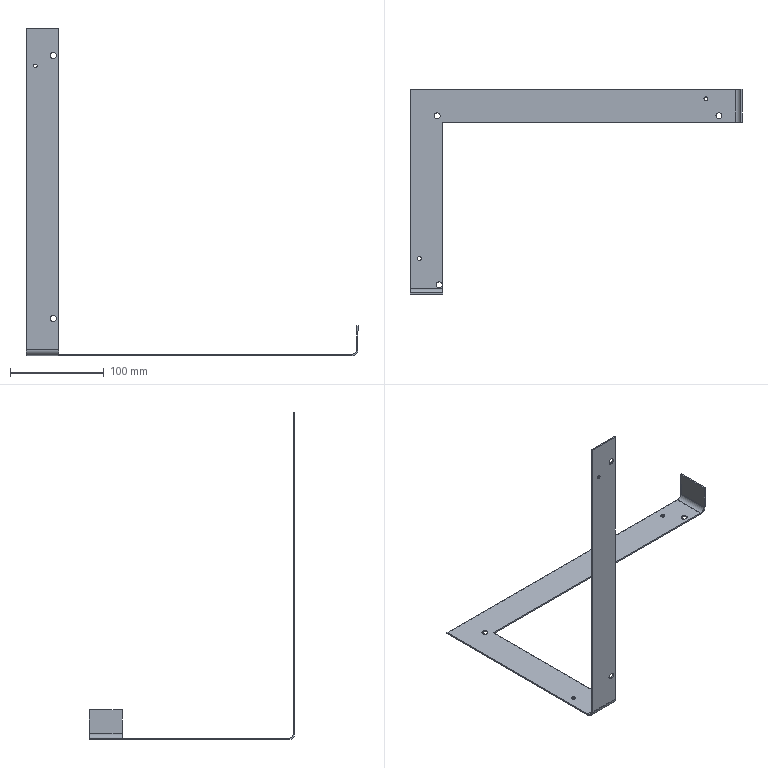Part | SolidWorks | features Cut 5, EdgeFlange 2, FlatPattern 1, SMBaseFlange 1, SheetMetal 1 | 1 solid | 40 faces | box 353.5 x 218.5 x 348.5 mm | volume 47454 mm3 | cylinder 20 | plane 20 | commonest cylinder face diameters 6.4 x10 4 x6 10 x2 13 x2
STEP:
#1=CARTESIAN_POINT('',(510.473,-27.361,-1.5));
#2=VERTEX_POINT('',#1);
#3=CARTESIAN_POINT('',(516.873,-27.361,-1.5));
#4=VERTEX_POINT('',#3);
#5=CARTESIAN_POINT('',(513.673,-27.361,-1.5));
#6=DIRECTION('',(0.,0.,1.));
#7=DIRECTION('',(1.,0.,0.));
#8=AXIS2_PLACEMENT_3D('',#5,#6,#7);
#9=CIRCLE('',#8,3.2);
#10=EDGE_CURVE('',#2,#4,#9,.T.);
#11=ORIENTED_EDGE('',*,*,#10,.F.);
#12=CARTESIAN_POINT('',(510.473,-27.361,0.));
#13=VERTEX_POINT('',#12);
#14=CARTESIAN_POINT('',(510.473,-27.361,-1.5));
#15=DIRECTION('',(0.,0.,1.));
#16=VECTOR('',#15,1000.);
#17=LINE('',#14,#16);
#18=EDGE_CURVE('',#2,#13,#17,.T.);
#19=ORIENTED_EDGE('',*,*,#18,.T.);
#20=CARTESIAN_POINT('',(516.873,-27.361,0.));
#21=VERTEX_POINT('',#20);
#22=CARTESIAN_POINT('',(513.673,-27.361,0.));
#23=DIRECTION('',(0.,0.,1.));
#24=DIRECTION('',(1.,0.,0.));
#25=AXIS2_PLACEMENT_3D('',#22,#23,#24);
#26=CIRCLE('',#25,3.2);
#27=EDGE_CURVE('',#13,#21,#26,.T.);
#28=ORIENTED_EDGE('',*,*,#27,.T.);
#29=CARTESIAN_POINT('',(516.873,-27.361,-1.5));
#30=DIRECTION('',(0.,0.,1.));
#31=VECTOR('',#30,1000.);
#32=LINE('',#29,#31);
#33=EDGE_CURVE('',#4,#21,#32,.T.);
#34=ORIENTED_EDGE('',*,*,#33,.F.);
#35=EDGE_LOOP('',(#11,#19,#28,#34));
#36=FACE_OUTER_BOUND('',#35,.T.);
#37=CARTESIAN_POINT('',(513.673,-27.361,-1.5));
#38=DIRECTION('',(0.,0.,1.));
#39=DIRECTION('',(1.,0.,0.));
#40=AXIS2_PLACEMENT_3D('',#37,#38,#39);
#41=CYLINDRICAL_SURFACE('',#40,3.2);
#42=ADVANCED_FACE('',(#36),#41,.F.);
#43=CARTESIAN_POINT('',(213.673,-217.715,314.8));
#44=VERTEX_POINT('',#43);
#45=CARTESIAN_POINT('',(213.673,-217.715,321.2));
#46=VERTEX_POINT('',#45);
#47=CARTESIAN_POINT('',(213.673,-217.715,318.));
#48=DIRECTION('',(0.,1.,0.));
#49=DIRECTION('',(0.,0.,1.));
#50=AXIS2_PLACEMENT_3D('',#47,#48,#49);
#51=CIRCLE('',#50,3.2);
#52=EDGE_CURVE('',#44,#46,#51,.T.);
#53=ORIENTED_EDGE('',*,*,#52,.F.);
#54=CARTESIAN_POINT('',(213.673,-216.215,314.8));
#55=VERTEX_POINT('',#54);
#56=CARTESIAN_POINT('',(213.673,-217.715,314.8));
#57=DIRECTION('',(0.,1.,0.));
#58=VECTOR('',#57,1000.);
#59=LINE('',#56,#58);
#60=EDGE_CURVE('',#44,#55,#59,.T.);
#61=ORIENTED_EDGE('',*,*,#60,.T.);
#62=CARTESIAN_POINT('',(213.673,-216.215,321.2));
#63=VERTEX_POINT('',#62);
#64=CARTESIAN_POINT('',(213.673,-216.215,318.));
#65=DIRECTION('',(0.,1.,0.));
#66=DIRECTION('',(0.,0.,1.));
#67=AXIS2_PLACEMENT_3D('',#64,#65,#66);
#68=CIRCLE('',#67,3.2);
#69=EDGE_CURVE('',#55,#63,#68,.T.);
#70=ORIENTED_EDGE('',*,*,#69,.T.);
#71=CARTESIAN_POINT('',(213.673,-217.715,321.2));
#72=DIRECTION('',(0.,1.,0.));
#73=VECTOR('',#72,1000.);
#74=LINE('',#71,#73);
#75=EDGE_CURVE('',#46,#63,#74,.T.);
#76=ORIENTED_EDGE('',*,*,#75,.F.);
#77=EDGE_LOOP('',(#53,#61,#70,#76));
#78=FACE_OUTER_BOUND('',#77,.T.);
#79=CARTESIAN_POINT('',(213.673,-217.715,318.));
#80=DIRECTION('',(0.,1.,0.));
#81=DIRECTION('',(0.,0.,1.));
#82=AXIS2_PLACEMENT_3D('',#79,#80,#81);
#83=CYLINDRICAL_SURFACE('',#82,3.2);
#84=ADVANCED_FACE('',(#78),#83,.F.);
#85=CARTESIAN_POINT('',(213.673,-217.715,34.8));
#86=VERTEX_POINT('',#85);
#87=CARTESIAN_POINT('',(213.673,-217.715,41.2));
#88=VERTEX_POINT('',#87);
#89=CARTESIAN_POINT('',(213.673,-217.715,38.));
#90=DIRECTION('',(0.,1.,0.));
#91=DIRECTION('',(0.,0.,1.));
#92=AXIS2_PLACEMENT_3D('',#89,#90,#91);
#93=CIRCLE('',#92,3.2);
#94=EDGE_CURVE('',#86,#88,#93,.T.);
#95=ORIENTED_EDGE('',*,*,#94,.F.);
#96=CARTESIAN_POINT('',(213.673,-216.215,34.8));
#97=VERTEX_POINT('',#96);
#98=CARTESIAN_POINT('',(213.673,-217.715,34.8));
#99=DIRECTION('',(0.,1.,0.));
#100=VECTOR('',#99,1000.);
#101=LINE('',#98,#100);
#102=EDGE_CURVE('',#86,#97,#101,.T.);
#103=ORIENTED_EDGE('',*,*,#102,.T.);
#104=CARTESIAN_POINT('',(213.673,-216.215,41.2));
#105=VERTEX_POINT('',#104);
#106=CARTESIAN_POINT('',(213.673,-216.215,38.));
#107=DIRECTION('',(0.,1.,0.));
#108=DIRECTION('',(0.,0.,1.));
#109=AXIS2_PLACEMENT_3D('',#106,#107,#108);
#110=CIRCLE('',#109,3.2);
#111=EDGE_CURVE('',#97,#105,#110,.T.);
#112=ORIENTED_EDGE('',*,*,#111,.T.);
#113=CARTESIAN_POINT('',(213.673,-217.715,41.2));
#114=DIRECTION('',(0.,1.,0.));
#115=VECTOR('',#114,1000.);
#116=LINE('',#113,#115);
#117=EDGE_CURVE('',#88,#105,#116,.T.);
#118=ORIENTED_EDGE('',*,*,#117,.F.);
#119=EDGE_LOOP('',(#95,#103,#112,#118));
#120=FACE_OUTER_BOUND('',#119,.T.);
#121=CARTESIAN_POINT('',(213.673,-217.715,38.));
#122=DIRECTION('',(0.,1.,0.));
#123=DIRECTION('',(0.,0.,1.));
#124=AXIS2_PLACEMENT_3D('',#121,#122,#123);
#125=CYLINDRICAL_SURFACE('',#124,3.2);
#126=ADVANCED_FACE('',(#120),#125,.F.);
#127=CARTESIAN_POINT('',(212.473,-207.35,-1.5));
#128=VERTEX_POINT('',#127);
#129=CARTESIAN_POINT('',(218.873,-207.35,-1.5));
#130=VERTEX_POINT('',#129);
#131=CARTESIAN_POINT('',(215.673,-207.35,-1.5));
#132=DIRECTION('',(0.,0.,1.));
#133=DIRECTION('',(1.,0.,0.));
#134=AXIS2_PLACEMENT_3D('',#131,#132,#133);
#135=CIRCLE('',#134,3.2);
#136=EDGE_CURVE('',#128,#130,#135,.T.);
#137=ORIENTED_EDGE('',*,*,#136,.F.);
#138=CARTESIAN_POINT('',(212.473,-207.35,0.));
#139=VERTEX_POINT('',#138);
#140=CARTESIAN_POINT('',(212.473,-207.35,-1.5));
#141=DIRECTION('',(0.,0.,1.));
#142=VECTOR('',#141,1000.);
#143=LINE('',#140,#142);
#144=EDGE_CURVE('',#128,#139,#143,.T.);
#145=ORIENTED_EDGE('',*,*,#144,.T.);
#146=CARTESIAN_POINT('',(218.873,-207.35,0.));
#147=VERTEX_POINT('',#146);
#148=CARTESIAN_POINT('',(215.673,-207.35,0.));
#149=DIRECTION('',(0.,0.,1.));
#150=DIRECTION('',(1.,0.,0.));
#151=AXIS2_PLACEMENT_3D('',#148,#149,#150);
#152=CIRCLE('',#151,3.2);
#153=EDGE_CURVE('',#139,#147,#152,.T.);
#154=ORIENTED_EDGE('',*,*,#153,.T.);
#155=CARTESIAN_POINT('',(218.873,-207.35,-1.5));
#156=DIRECTION('',(0.,0.,1.));
#157=VECTOR('',#156,1000.);
#158=LINE('',#155,#157);
#159=EDGE_CURVE('',#130,#147,#158,.T.);
#160=ORIENTED_EDGE('',*,*,#159,.F.);
#161=EDGE_LOOP('',(#137,#145,#154,#160));
#162=FACE_OUTER_BOUND('',#161,.T.);
#163=CARTESIAN_POINT('',(215.673,-207.35,-1.5));
#164=DIRECTION('',(0.,0.,1.));
#165=DIRECTION('',(1.,0.,0.));
#166=AXIS2_PLACEMENT_3D('',#163,#164,#165);
#167=CYLINDRICAL_SURFACE('',#166,3.2);
#168=ADVANCED_FACE('',(#162),#167,.F.);
#169=CARTESIAN_POINT('',(210.473,-27.361,-1.5));
#170=VERTEX_POINT('',#169);
#171=CARTESIAN_POINT('',(216.873,-27.361,-1.5));
#172=VERTEX_POINT('',#171);
#173=CARTESIAN_POINT('',(213.673,-27.361,-1.5));
#174=DIRECTION('',(0.,0.,1.));
#175=DIRECTION('',(1.,0.,0.));
#176=AXIS2_PLACEMENT_3D('',#173,#174,#175);
#177=CIRCLE('',#176,3.2);
#178=EDGE_CURVE('',#170,#172,#177,.T.);
#179=ORIENTED_EDGE('',*,*,#178,.F.);
#180=CARTESIAN_POINT('',(210.473,-27.361,0.));
#181=VERTEX_POINT('',#180);
#182=CARTESIAN_POINT('',(210.473,-27.361,-1.5));
#183=DIRECTION('',(0.,0.,1.));
#184=VECTOR('',#183,1000.);
#185=LINE('',#182,#184);
#186=EDGE_CURVE('',#170,#181,#185,.T.);
#187=ORIENTED_EDGE('',*,*,#186,.T.);
#188=CARTESIAN_POINT('',(216.873,-27.361,0.));
#189=VERTEX_POINT('',#188);
#190=CARTESIAN_POINT('',(213.673,-27.361,0.));
#191=DIRECTION('',(0.,0.,1.));
#192=DIRECTION('',(1.,0.,0.));
#193=AXIS2_PLACEMENT_3D('',#190,#191,#192);
#194=CIRCLE('',#193,3.2);
#195=EDGE_CURVE('',#181,#189,#194,.T.);
#196=ORIENTED_EDGE('',*,*,#195,.T.);
#197=CARTESIAN_POINT('',(216.873,-27.361,-1.5));
#198=DIRECTION('',(0.,0.,1.));
#199=VECTOR('',#198,1000.);
#200=LINE('',#197,#199);
#201=EDGE_CURVE('',#172,#189,#200,.T.);
#202=ORIENTED_EDGE('',*,*,#201,.F.);
#203=EDGE_LOOP('',(#179,#187,#196,#202));
#204=FACE_OUTER_BOUND('',#203,.T.);
#205=CARTESIAN_POINT('',(213.673,-27.361,-1.5));
#206=DIRECTION('',(0.,0.,1.));
#207=DIRECTION('',(1.,0.,0.));
#208=AXIS2_PLACEMENT_3D('',#205,#206,#207);
#209=CYLINDRICAL_SURFACE('',#208,3.2);
#210=ADVANCED_FACE('',(#204),#209,.F.);
#211=CARTESIAN_POINT('',(194.673,-216.215,305.));
#212=VERTEX_POINT('',#211);
#213=CARTESIAN_POINT('',(194.673,-216.215,309.));
#214=VERTEX_POINT('',#213);
#215=CARTESIAN_POINT('',(194.673,-216.215,307.));
#216=DIRECTION('',(0.,1.,0.));
#217=DIRECTION('',(0.,0.,1.));
#218=AXIS2_PLACEMENT_3D('',#215,#216,#217);
#219=CIRCLE('',#218,2.);
#220=EDGE_CURVE('',#212,#214,#219,.T.);
#221=ORIENTED_EDGE('',*,*,#220,.T.);
#222=CARTESIAN_POINT('',(194.673,-217.715,309.));
#223=VERTEX_POINT('',#222);
#224=CARTESIAN_POINT('',(194.673,-207.715,309.));
#225=DIRECTION('',(0.,-1.,0.));
#226=VECTOR('',#225,1000.);
#227=LINE('',#224,#226);
#228=EDGE_CURVE('',#214,#223,#227,.T.);
#229=ORIENTED_EDGE('',*,*,#228,.T.);
#230=CARTESIAN_POINT('',(194.673,-217.715,305.));
#231=VERTEX_POINT('',#230);
#232=CARTESIAN_POINT('',(194.673,-217.715,307.));
#233=DIRECTION('',(0.,-1.,0.));
#234=DIRECTION('',(0.,0.,-1.));
#235=AXIS2_PLACEMENT_3D('',#232,#233,#234);
#236=CIRCLE('',#235,2.);
#237=EDGE_CURVE('',#223,#231,#236,.T.);
#238=ORIENTED_EDGE('',*,*,#237,.T.);
#239=CARTESIAN_POINT('',(194.673,-207.715,305.));
#240=DIRECTION('',(0.,-1.,0.));
#241=VECTOR('',#240,1000.);
#242=LINE('',#239,#241);
#243=EDGE_CURVE('',#212,#231,#242,.T.);
#244=ORIENTED_EDGE('',*,*,#243,.F.);
#245=EDGE_LOOP('',(#221,#229,#238,#244));
#246=FACE_OUTER_BOUND('',#245,.T.);
#247=CARTESIAN_POINT('',(194.673,-207.715,307.));
#248=DIRECTION('',(0.,-1.,0.));
#249=DIRECTION('',(0.,0.,-1.));
#250=AXIS2_PLACEMENT_3D('',#247,#248,#249);
#251=CYLINDRICAL_SURFACE('',#250,2.);
#252=ADVANCED_FACE('',(#246),#251,.F.);
#253=CARTESIAN_POINT('',(497.673,-9.215,0.));
#254=VERTEX_POINT('',#253);
#255=CARTESIAN_POINT('',(501.673,-9.215,0.));
#256=VERTEX_POINT('',#255);
#257=CARTESIAN_POINT('',(499.673,-9.215,0.));
#258=DIRECTION('',(0.,0.,1.));
#259=DIRECTION('',(1.,0.,0.));
#260=AXIS2_PLACEMENT_3D('',#257,#258,#259);
#261=CIRCLE('',#260,2.);
#262=EDGE_CURVE('',#254,#256,#261,.T.);
#263=ORIENTED_EDGE('',*,*,#262,.T.);
#264=CARTESIAN_POINT('',(501.673,-9.215,-1.5));
#265=VERTEX_POINT('',#264);
#266=CARTESIAN_POINT('',(501.673,-9.215,8.5));
#267=DIRECTION('',(0.,0.,-1.));
#268=VECTOR('',#267,1000.);
#269=LINE('',#266,#268);
#270=EDGE_CURVE('',#256,#265,#269,.T.);
#271=ORIENTED_EDGE('',*,*,#270,.T.);
#272=CARTESIAN_POINT('',(497.673,-9.215,-1.5));
#273=VERTEX_POINT('',#272);
#274=CARTESIAN_POINT('',(499.673,-9.215,-1.5));
#275=DIRECTION('',(0.,0.,-1.));
#276=DIRECTION('',(-1.,0.,0.));
#277=AXIS2_PLACEMENT_3D('',#274,#275,#276);
#278=CIRCLE('',#277,2.);
#279=EDGE_CURVE('',#265,#273,#278,.T.);
#280=ORIENTED_EDGE('',*,*,#279,.T.);
#281=CARTESIAN_POINT('',(497.673,-9.215,8.5));
#282=DIRECTION('',(0.,0.,-1.));
#283=VECTOR('',#282,1000.);
#284=LINE('',#281,#283);
#285=EDGE_CURVE('',#254,#273,#284,.T.);
#286=ORIENTED_EDGE('',*,*,#285,.F.);
#287=EDGE_LOOP('',(#263,#271,#280,#286));
#288=FACE_OUTER_BOUND('',#287,.T.);
#289=CARTESIAN_POINT('',(499.673,-9.215,8.5));
#290=DIRECTION('',(0.,0.,-1.));
#291=DIRECTION('',(-1.,0.,0.));
#292=AXIS2_PLACEMENT_3D('',#289,#290,#291);
#293=CYLINDRICAL_SURFACE('',#292,2.);
#294=ADVANCED_FACE('',(#288),#293,.F.);
#295=CARTESIAN_POINT('',(192.673,-179.215,0.));
#296=VERTEX_POINT('',#295);
#297=CARTESIAN_POINT('',(196.673,-179.215,0.));
#298=VERTEX_POINT('',#297);
#299=CARTESIAN_POINT('',(194.673,-179.215,0.));
#300=DIRECTION('',(0.,0.,1.));
#301=DIRECTION('',(1.,0.,0.));
#302=AXIS2_PLACEMENT_3D('',#299,#300,#301);
#303=CIRCLE('',#302,2.);
#304=EDGE_CURVE('',#296,#298,#303,.T.);
#305=ORIENTED_EDGE('',*,*,#304,.T.);
#306=CARTESIAN_POINT('',(196.673,-179.215,-1.5));
#307=VERTEX_POINT('',#306);
#308=CARTESIAN_POINT('',(196.673,-179.215,8.5));
#309=DIRECTION('',(0.,0.,-1.));
#310=VECTOR('',#309,1000.);
#311=LINE('',#308,#310);
#312=EDGE_CURVE('',#298,#307,#311,.T.);
#313=ORIENTED_EDGE('',*,*,#312,.T.);
#314=CARTESIAN_POINT('',(192.673,-179.215,-1.5));
#315=VERTEX_POINT('',#314);
#316=CARTESIAN_POINT('',(194.673,-179.215,-1.5));
#317=DIRECTION('',(0.,0.,-1.));
#318=DIRECTION('',(-1.,0.,0.));
#319=AXIS2_PLACEMENT_3D('',#316,#317,#318);
#320=CIRCLE('',#319,2.);
#321=EDGE_CURVE('',#307,#315,#320,.T.);
#322=ORIENTED_EDGE('',*,*,#321,.T.);
#323=CARTESIAN_POINT('',(192.673,-179.215,8.5));
#324=DIRECTION('',(0.,0.,-1.));
#325=VECTOR('',#324,1000.);
#326=LINE('',#323,#325);
#327=EDGE_CURVE('',#296,#315,#326,.T.);
#328=ORIENTED_EDGE('',*,*,#327,.F.);
#329=EDGE_LOOP('',(#305,#313,#322,#328));
#330=FACE_OUTER_BOUND('',#329,.T.);
#331=CARTESIAN_POINT('',(194.673,-179.215,8.5));
#332=DIRECTION('',(0.,0.,-1.));
#333=DIRECTION('',(-1.,0.,0.));
#334=AXIS2_PLACEMENT_3D('',#331,#332,#333);
#335=CYLINDRICAL_SURFACE('',#334,2.);
#336=ADVANCED_FACE('',(#330),#335,.F.);
#337=CARTESIAN_POINT('',(513.673,-27.361,-1.5));
#338=DIRECTION('',(0.,0.,1.));
#339=DIRECTION('',(1.,0.,0.));
#340=AXIS2_PLACEMENT_3D('',#337,#338,#339);
#341=CIRCLE('',#340,3.2);
#342=EDGE_CURVE('',#4,#2,#341,.T.);
#343=ORIENTED_EDGE('',*,*,#342,.T.);
#344=ORIENTED_EDGE('',*,*,#10,.T.);
#345=EDGE_LOOP('',(#343,#344));
#346=FACE_BOUND('',#345,.T.);
#347=CARTESIAN_POINT('',(215.673,-207.35,-1.5));
#348=DIRECTION('',(0.,0.,1.));
#349=DIRECTION('',(1.,0.,0.));
#350=AXIS2_PLACEMENT_3D('',#347,#348,#349);
#351=CIRCLE('',#350,3.2);
#352=EDGE_CURVE('',#130,#128,#351,.T.);
#353=ORIENTED_EDGE('',*,*,#352,.T.);
#354=ORIENTED_EDGE('',*,*,#136,.T.);
#355=EDGE_LOOP('',(#353,#354));
#356=FACE_BOUND('',#355,.T.);
#357=CARTESIAN_POINT('',(213.673,-27.361,-1.5));
#358=DIRECTION('',(0.,0.,1.));
#359=DIRECTION('',(1.,0.,0.));
#360=AXIS2_PLACEMENT_3D('',#357,#358,#359);
#361=CIRCLE('',#360,3.2);
#362=EDGE_CURVE('',#172,#170,#361,.T.);
#363=ORIENTED_EDGE('',*,*,#362,.T.);
#364=ORIENTED_EDGE('',*,*,#178,.T.);
#365=EDGE_LOOP('',(#363,#364));
#366=FACE_BOUND('',#365,.T.);
#367=CARTESIAN_POINT('',(499.673,-9.215,-1.5));
#368=DIRECTION('',(0.,0.,-1.));
#369=DIRECTION('',(-1.,0.,0.));
#370=AXIS2_PLACEMENT_3D('',#367,#368,#369);
#371=CIRCLE('',#370,2.);
#372=EDGE_CURVE('',#273,#265,#371,.T.);
#373=ORIENTED_EDGE('',*,*,#372,.F.);
#374=ORIENTED_EDGE('',*,*,#279,.F.);
#375=EDGE_LOOP('',(#373,#374));
#376=FACE_BOUND('',#375,.T.);
#377=CARTESIAN_POINT('',(194.673,-179.215,-1.5));
#378=DIRECTION('',(0.,0.,-1.));
#379=DIRECTION('',(-1.,0.,0.));
#380=AXIS2_PLACEMENT_3D('',#377,#378,#379);
#381=CIRCLE('',#380,2.);
#382=EDGE_CURVE('',#315,#307,#381,.T.);
#383=ORIENTED_EDGE('',*,*,#382,.F.);
#384=ORIENTED_EDGE('',*,*,#321,.F.);
#385=EDGE_LOOP('',(#383,#384));
#386=FACE_BOUND('',#385,.T.);
#387=CARTESIAN_POINT('',(531.673,0.7853,-1.5));
#388=VERTEX_POINT('',#387);
#389=CARTESIAN_POINT('',(531.673,-34.215,-1.5));
#390=VERTEX_POINT('',#389);
#391=CARTESIAN_POINT('',(531.673,0.7853,-1.5));
#392=DIRECTION('',(0.,-1.,0.));
#393=VECTOR('',#392,1000.);
#394=LINE('',#391,#393);
#395=EDGE_CURVE('',#388,#390,#394,.T.);
#396=ORIENTED_EDGE('',*,*,#395,.T.);
#397=CARTESIAN_POINT('',(219.673,-34.215,-1.5));
#398=VERTEX_POINT('',#397);
#399=CARTESIAN_POINT('',(219.673,-34.215,-1.5));
#400=DIRECTION('',(1.,0.,0.));
#401=VECTOR('',#400,1000.);
#402=LINE('',#399,#401);
#403=EDGE_CURVE('',#398,#390,#402,.T.);
#404=ORIENTED_EDGE('',*,*,#403,.F.);
#405=CARTESIAN_POINT('',(219.673,-211.215,-1.5));
#406=VERTEX_POINT('',#405);
#407=CARTESIAN_POINT('',(219.673,-34.215,-1.5));
#408=DIRECTION('',(0.,1.,0.));
#409=VECTOR('',#408,1000.);
#410=LINE('',#407,#409);
#411=EDGE_CURVE('',#406,#398,#410,.T.);
#412=ORIENTED_EDGE('',*,*,#411,.F.);
#413=CARTESIAN_POINT('',(184.673,-211.215,-1.5));
#414=VERTEX_POINT('',#413);
#415=CARTESIAN_POINT('',(219.673,-211.215,-1.5));
#416=DIRECTION('',(-1.,0.,0.));
#417=VECTOR('',#416,1000.);
#418=LINE('',#415,#417);
#419=EDGE_CURVE('',#406,#414,#418,.T.);
#420=ORIENTED_EDGE('',*,*,#419,.T.);
#421=CARTESIAN_POINT('',(184.673,0.7853,-1.5));
#422=VERTEX_POINT('',#421);
#423=CARTESIAN_POINT('',(184.673,0.7853,-1.5));
#424=DIRECTION('',(0.,-1.,0.));
#425=VECTOR('',#424,1000.);
#426=LINE('',#423,#425);
#427=EDGE_CURVE('',#422,#414,#426,.T.);
#428=ORIENTED_EDGE('',*,*,#427,.F.);
#429=CARTESIAN_POINT('',(184.673,0.7853,-1.5));
#430=DIRECTION('',(-1.,0.,0.));
#431=VECTOR('',#430,1000.);
#432=LINE('',#429,#431);
#433=EDGE_CURVE('',#388,#422,#432,.T.);
#434=ORIENTED_EDGE('',*,*,#433,.F.);
#435=EDGE_LOOP('',(#396,#404,#412,#420,#428,#434));
#436=FACE_OUTER_BOUND('',#435,.T.);
#437=CARTESIAN_POINT('',(0.,0.,-1.5));
#438=DIRECTION('',(0.,0.,1.));
#439=DIRECTION('',(1.,0.,0.));
#440=AXIS2_PLACEMENT_3D('',#437,#438,#439);
#441=PLANE('',#440);
#442=ADVANCED_FACE('',(#346,#356,#366,#376,#386,#436),#441,.F.);
#443=CARTESIAN_POINT('',(513.673,-27.361,0.));
#444=DIRECTION('',(0.,0.,1.));
#445=DIRECTION('',(1.,0.,0.));
#446=AXIS2_PLACEMENT_3D('',#443,#444,#445);
#447=CIRCLE('',#446,3.2);
#448=EDGE_CURVE('',#21,#13,#447,.T.);
#449=ORIENTED_EDGE('',*,*,#448,.F.);
#450=ORIENTED_EDGE('',*,*,#27,.F.);
#451=EDGE_LOOP('',(#449,#450));
#452=FACE_BOUND('',#451,.T.);
#453=CARTESIAN_POINT('',(215.673,-207.35,0.));
#454=DIRECTION('',(0.,0.,1.));
#455=DIRECTION('',(1.,0.,0.));
#456=AXIS2_PLACEMENT_3D('',#453,#454,#455);
#457=CIRCLE('',#456,3.2);
#458=EDGE_CURVE('',#147,#139,#457,.T.);
#459=ORIENTED_EDGE('',*,*,#458,.F.);
#460=ORIENTED_EDGE('',*,*,#153,.F.);
#461=EDGE_LOOP('',(#459,#460));
#462=FACE_BOUND('',#461,.T.);
#463=CARTESIAN_POINT('',(213.673,-27.361,0.));
#464=DIRECTION('',(0.,0.,1.));
#465=DIRECTION('',(1.,0.,0.));
#466=AXIS2_PLACEMENT_3D('',#463,#464,#465);
#467=CIRCLE('',#466,3.2);
#468=EDGE_CURVE('',#189,#181,#467,.T.);
#469=ORIENTED_EDGE('',*,*,#468,.F.);
#470=ORIENTED_EDGE('',*,*,#195,.F.);
#471=EDGE_LOOP('',(#469,#470));
#472=FACE_BOUND('',#471,.T.);
#473=ORIENTED_EDGE('',*,*,#262,.F.);
#474=CARTESIAN_POINT('',(499.673,-9.215,0.));
#475=DIRECTION('',(0.,0.,1.));
#476=DIRECTION('',(1.,0.,0.));
#477=AXIS2_PLACEMENT_3D('',#474,#475,#476);
#478=CIRCLE('',#477,2.);
#479=EDGE_CURVE('',#256,#254,#478,.T.);
#480=ORIENTED_EDGE('',*,*,#479,.F.);
#481=EDGE_LOOP('',(#473,#480));
#482=FACE_BOUND('',#481,.T.);
#483=ORIENTED_EDGE('',*,*,#304,.F.);
#484=CARTESIAN_POINT('',(194.673,-179.215,0.));
#485=DIRECTION('',(0.,0.,1.));
#486=DIRECTION('',(1.,0.,0.));
#487=AXIS2_PLACEMENT_3D('',#484,#485,#486);
#488=CIRCLE('',#487,2.);
#489=EDGE_CURVE('',#298,#296,#488,.T.);
#490=ORIENTED_EDGE('',*,*,#489,.F.);
#491=EDGE_LOOP('',(#483,#490));
#492=FACE_BOUND('',#491,.T.);
#493=CARTESIAN_POINT('',(219.673,-34.215,0.));
#494=VERTEX_POINT('',#493);
#495=CARTESIAN_POINT('',(531.673,-34.215,0.));
#496=VERTEX_POINT('',#495);
#497=CARTESIAN_POINT('',(219.673,-34.215,0.));
#498=DIRECTION('',(1.,0.,0.));
#499=VECTOR('',#498,1000.);
#500=LINE('',#497,#499);
#501=EDGE_CURVE('',#494,#496,#500,.T.);
#502=ORIENTED_EDGE('',*,*,#501,.T.);
#503=CARTESIAN_POINT('',(531.673,0.7853,0.));
#504=VERTEX_POINT('',#503);
#505=CARTESIAN_POINT('',(531.673,0.7853,0.));
#506=DIRECTION('',(0.,-1.,0.));
#507=VECTOR('',#506,1000.);
#508=LINE('',#505,#507);
#509=EDGE_CURVE('',#504,#496,#508,.T.);
#510=ORIENTED_EDGE('',*,*,#509,.F.);
#511=CARTESIAN_POINT('',(184.673,0.7853,0.));
#512=VERTEX_POINT('',#511);
#513=CARTESIAN_POINT('',(184.673,0.7853,0.));
#514=DIRECTION('',(-1.,0.,0.));
#515=VECTOR('',#514,1000.);
#516=LINE('',#513,#515);
#517=EDGE_CURVE('',#504,#512,#516,.T.);
#518=ORIENTED_EDGE('',*,*,#517,.T.);
#519=CARTESIAN_POINT('',(184.673,-211.215,0.));
#520=VERTEX_POINT('',#519);
#521=CARTESIAN_POINT('',(184.673,0.7853,0.));
#522=DIRECTION('',(0.,-1.,0.));
#523=VECTOR('',#522,1000.);
#524=LINE('',#521,#523);
#525=EDGE_CURVE('',#512,#520,#524,.T.);
#526=ORIENTED_EDGE('',*,*,#525,.T.);
#527=CARTESIAN_POINT('',(219.673,-211.215,0.));
#528=VERTEX_POINT('',#527);
#529=CARTESIAN_POINT('',(219.673,-211.215,0.));
#530=DIRECTION('',(-1.,0.,0.));
#531=VECTOR('',#530,1000.);
#532=LINE('',#529,#531);
#533=EDGE_CURVE('',#528,#520,#532,.T.);
#534=ORIENTED_EDGE('',*,*,#533,.F.);
#535=CARTESIAN_POINT('',(219.673,-34.215,0.));
#536=DIRECTION('',(0.,1.,0.));
#537=VECTOR('',#536,1000.);
#538=LINE('',#535,#537);
#539=EDGE_CURVE('',#528,#494,#538,.T.);
#540=ORIENTED_EDGE('',*,*,#539,.T.);
#541=EDGE_LOOP('',(#502,#510,#518,#526,#534,#540));
#542=FACE_OUTER_BOUND('',#541,.T.);
#543=CARTESIAN_POINT('',(0.,0.,0.));
#544=DIRECTION('',(0.,0.,1.));
#545=DIRECTION('',(1.,0.,0.));
#546=AXIS2_PLACEMENT_3D('',#543,#544,#545);
#547=PLANE('',#546);
#548=ADVANCED_FACE('',(#452,#462,#472,#482,#492,#542),#547,.T.);
#549=ORIENTED_EDGE('',*,*,#517,.F.);
#550=CARTESIAN_POINT('',(531.673,0.7853,0.));
#551=DIRECTION('',(0.,0.,-1.));
#552=VECTOR('',#551,1000.);
#553=LINE('',#550,#552);
#554=EDGE_CURVE('',#504,#388,#553,.T.);
#555=ORIENTED_EDGE('',*,*,#554,.T.);
#556=ORIENTED_EDGE('',*,*,#433,.T.);
#557=CARTESIAN_POINT('',(184.673,0.7853,-1.5));
#558=DIRECTION('',(0.,0.,1.));
#559=VECTOR('',#558,1000.);
#560=LINE('',#557,#559);
#561=EDGE_CURVE('',#422,#512,#560,.T.);
#562=ORIENTED_EDGE('',*,*,#561,.T.);
#563=EDGE_LOOP('',(#549,#555,#556,#562));
#564=FACE_OUTER_BOUND('',#563,.T.);
#565=CARTESIAN_POINT('',(184.673,0.7853,-1.5));
#566=DIRECTION('',(0.,1.,0.));
#567=DIRECTION('',(0.,0.,1.));
#568=AXIS2_PLACEMENT_3D('',#565,#566,#567);
#569=PLANE('',#568);
#570=ADVANCED_FACE('',(#564),#569,.T.);
#571=ORIENTED_EDGE('',*,*,#539,.F.);
#572=CARTESIAN_POINT('',(219.673,-211.215,0.));
#573=DIRECTION('',(0.,0.,-1.));
#574=VECTOR('',#573,1000.);
#575=LINE('',#572,#574);
#576=EDGE_CURVE('',#528,#406,#575,.T.);
#577=ORIENTED_EDGE('',*,*,#576,.T.);
#578=ORIENTED_EDGE('',*,*,#411,.T.);
#579=CARTESIAN_POINT('',(219.673,-34.215,-1.5));
#580=DIRECTION('',(0.,0.,1.));
#581=VECTOR('',#580,1000.);
#582=LINE('',#579,#581);
#583=EDGE_CURVE('',#398,#494,#582,.T.);
#584=ORIENTED_EDGE('',*,*,#583,.T.);
#585=EDGE_LOOP('',(#571,#577,#578,#584));
#586=FACE_OUTER_BOUND('',#585,.T.);
#587=CARTESIAN_POINT('',(219.673,-34.215,-1.5));
#588=DIRECTION('',(1.,0.,0.));
#589=DIRECTION('',(0.,1.,0.));
#590=AXIS2_PLACEMENT_3D('',#587,#588,#589);
#591=PLANE('',#590);
#592=ADVANCED_FACE('',(#586),#591,.T.);
#593=CARTESIAN_POINT('',(184.673,-211.215,0.));
#594=DIRECTION('',(0.,0.,-1.));
#595=VECTOR('',#594,1000.);
#596=LINE('',#593,#595);
#597=EDGE_CURVE('',#520,#414,#596,.T.);
#598=ORIENTED_EDGE('',*,*,#597,.F.);
#599=ORIENTED_EDGE('',*,*,#525,.F.);
#600=ORIENTED_EDGE('',*,*,#561,.F.);
#601=ORIENTED_EDGE('',*,*,#427,.T.);
#602=EDGE_LOOP('',(#598,#599,#600,#601));
#603=FACE_OUTER_BOUND('',#602,.T.);
#604=CARTESIAN_POINT('',(184.673,0.7853,-1.5));
#605=DIRECTION('',(-1.,0.,0.));
#606=DIRECTION('',(0.,-1.,0.));
#607=AXIS2_PLACEMENT_3D('',#604,#605,#606);
#608=PLANE('',#607);
#609=ADVANCED_FACE('',(#603),#608,.T.);
#610=CARTESIAN_POINT('',(531.673,-34.215,0.));
#611=DIRECTION('',(0.,0.,-1.));
#612=VECTOR('',#611,1000.);
#613=LINE('',#610,#612);
#614=EDGE_CURVE('',#496,#390,#613,.T.);
#615=ORIENTED_EDGE('',*,*,#614,.F.);
#616=ORIENTED_EDGE('',*,*,#501,.F.);
#617=ORIENTED_EDGE('',*,*,#583,.F.);
#618=ORIENTED_EDGE('',*,*,#403,.T.);
#619=EDGE_LOOP('',(#615,#616,#617,#618));
#620=FACE_OUTER_BOUND('',#619,.T.);
#621=CARTESIAN_POINT('',(219.673,-34.215,-1.5));
#622=DIRECTION('',(0.,-1.,0.));
#623=DIRECTION('',(0.,0.,-1.));
#624=AXIS2_PLACEMENT_3D('',#621,#622,#623);
#625=PLANE('',#624);
#626=ADVANCED_FACE('',(#620),#625,.T.);
#627=CARTESIAN_POINT('',(184.673,-216.215,5.));
#628=VERTEX_POINT('',#627);
#629=CARTESIAN_POINT('',(184.673,-217.715,5.));
#630=VERTEX_POINT('',#629);
#631=CARTESIAN_POINT('',(184.673,-217.715,5.));
#632=DIRECTION('',(0.,-1.,0.));
#633=VECTOR('',#632,1000.);
#634=LINE('',#631,#633);
#635=EDGE_CURVE('',#628,#630,#634,.T.);
#636=ORIENTED_EDGE('',*,*,#635,.F.);
#637=CARTESIAN_POINT('',(184.673,-211.215,5.));
#638=DIRECTION('',(-1.,0.,0.));
#639=DIRECTION('',(0.,0.,-1.));
#640=AXIS2_PLACEMENT_3D('',#637,#638,#639);
#641=CIRCLE('',#640,5.);
#642=EDGE_CURVE('',#520,#628,#641,.T.);
#643=ORIENTED_EDGE('',*,*,#642,.F.);
#644=ORIENTED_EDGE('',*,*,#597,.T.);
#645=CARTESIAN_POINT('',(184.673,-211.215,5.));
#646=DIRECTION('',(-1.,0.,0.));
#647=DIRECTION('',(0.,0.,-1.));
#648=AXIS2_PLACEMENT_3D('',#645,#646,#647);
#649=CIRCLE('',#648,6.5);
#650=EDGE_CURVE('',#414,#630,#649,.T.);
#651=ORIENTED_EDGE('',*,*,#650,.T.);
#652=EDGE_LOOP('',(#636,#643,#644,#651));
#653=FACE_OUTER_BOUND('',#652,.T.);
#654=CARTESIAN_POINT('',(184.673,-211.215,5.));
#655=DIRECTION('',(-1.,0.,0.));
#656=DIRECTION('',(0.,0.,1.));
#657=AXIS2_PLACEMENT_3D('',#654,#655,#656);
#658=PLANE('',#657);
#659=ADVANCED_FACE('',(#653),#658,.T.);
#660=CARTESIAN_POINT('',(219.673,-216.215,5.));
#661=VERTEX_POINT('',#660);
#662=CARTESIAN_POINT('',(219.673,-211.215,5.));
#663=DIRECTION('',(1.,0.,0.));
#664=DIRECTION('',(0.,0.,-1.));
#665=AXIS2_PLACEMENT_3D('',#662,#663,#664);
#666=CIRCLE('',#665,5.);
#667=EDGE_CURVE('',#661,#528,#666,.T.);
#668=ORIENTED_EDGE('',*,*,#667,.F.);
#669=CARTESIAN_POINT('',(219.673,-217.715,5.));
#670=VERTEX_POINT('',#669);
#671=CARTESIAN_POINT('',(219.673,-216.215,5.));
#672=DIRECTION('',(0.,-1.,0.));
#673=VECTOR('',#672,1000.);
#674=LINE('',#671,#673);
#675=EDGE_CURVE('',#661,#670,#674,.T.);
#676=ORIENTED_EDGE('',*,*,#675,.T.);
#677=CARTESIAN_POINT('',(219.673,-211.215,5.));
#678=DIRECTION('',(1.,0.,0.));
#679=DIRECTION('',(0.,0.,-1.));
#680=AXIS2_PLACEMENT_3D('',#677,#678,#679);
#681=CIRCLE('',#680,6.5);
#682=EDGE_CURVE('',#670,#406,#681,.T.);
#683=ORIENTED_EDGE('',*,*,#682,.T.);
#684=ORIENTED_EDGE('',*,*,#576,.F.);
#685=EDGE_LOOP('',(#668,#676,#683,#684));
#686=FACE_OUTER_BOUND('',#685,.T.);
#687=CARTESIAN_POINT('',(219.673,-211.215,5.));
#688=DIRECTION('',(-1.,0.,0.));
#689=DIRECTION('',(0.,0.,1.));
#690=AXIS2_PLACEMENT_3D('',#687,#688,#689);
#691=PLANE('',#690);
#692=ADVANCED_FACE('',(#686),#691,.F.);
#693=ORIENTED_EDGE('',*,*,#419,.F.);
#694=ORIENTED_EDGE('',*,*,#682,.F.);
#695=CARTESIAN_POINT('',(184.673,-217.715,5.));
#696=DIRECTION('',(-1.,0.,0.));
#697=VECTOR('',#696,1000.);
#698=LINE('',#695,#697);
#699=EDGE_CURVE('',#670,#630,#698,.T.);
#700=ORIENTED_EDGE('',*,*,#699,.T.);
#701=ORIENTED_EDGE('',*,*,#650,.F.);
#702=EDGE_LOOP('',(#693,#694,#700,#701));
#703=FACE_OUTER_BOUND('',#702,.T.);
#704=CARTESIAN_POINT('',(219.673,-211.215,5.));
#705=DIRECTION('',(1.,0.,0.));
#706=DIRECTION('',(0.,-1.,0.));
#707=AXIS2_PLACEMENT_3D('',#704,#705,#706);
#708=CYLINDRICAL_SURFACE('',#707,6.5);
#709=ADVANCED_FACE('',(#703),#708,.T.);
#710=ORIENTED_EDGE('',*,*,#533,.T.);
#711=ORIENTED_EDGE('',*,*,#642,.T.);
#712=CARTESIAN_POINT('',(184.673,-216.215,5.));
#713=DIRECTION('',(1.,0.,0.));
#714=VECTOR('',#713,1000.);
#715=LINE('',#712,#714);
#716=EDGE_CURVE('',#628,#661,#715,.T.);
#717=ORIENTED_EDGE('',*,*,#716,.T.);
#718=ORIENTED_EDGE('',*,*,#667,.T.);
#719=EDGE_LOOP('',(#710,#711,#717,#718));
#720=FACE_OUTER_BOUND('',#719,.T.);
#721=CARTESIAN_POINT('',(219.673,-211.215,5.));
#722=DIRECTION('',(1.,0.,0.));
#723=DIRECTION('',(0.,-1.,0.));
#724=AXIS2_PLACEMENT_3D('',#721,#722,#723);
#725=CYLINDRICAL_SURFACE('',#724,5.);
#726=ADVANCED_FACE('',(#720),#725,.F.);
#727=ORIENTED_EDGE('',*,*,#675,.F.);
#728=CARTESIAN_POINT('',(219.673,-216.215,347.));
#729=VERTEX_POINT('',#728);
#730=CARTESIAN_POINT('',(219.673,-216.215,347.));
#731=DIRECTION('',(0.,0.,1.));
#732=VECTOR('',#731,1000.);
#733=LINE('',#730,#732);
#734=EDGE_CURVE('',#661,#729,#733,.T.);
#735=ORIENTED_EDGE('',*,*,#734,.T.);
#736=CARTESIAN_POINT('',(219.673,-217.715,347.));
#737=VERTEX_POINT('',#736);
#738=CARTESIAN_POINT('',(219.673,-217.715,347.));
#739=DIRECTION('',(0.,1.,0.));
#740=VECTOR('',#739,1000.);
#741=LINE('',#738,#740);
#742=EDGE_CURVE('',#737,#729,#741,.T.);
#743=ORIENTED_EDGE('',*,*,#742,.F.);
#744=CARTESIAN_POINT('',(219.673,-217.715,0.));
#745=DIRECTION('',(0.,0.,1.));
#746=VECTOR('',#745,1000.);
#747=LINE('',#744,#746);
#748=EDGE_CURVE('',#670,#737,#747,.T.);
#749=ORIENTED_EDGE('',*,*,#748,.F.);
#750=EDGE_LOOP('',(#727,#735,#743,#749));
#751=FACE_OUTER_BOUND('',#750,.T.);
#752=CARTESIAN_POINT('',(219.673,-217.715,347.));
#753=DIRECTION('',(-1.,0.,0.));
#754=DIRECTION('',(0.,0.,1.));
#755=AXIS2_PLACEMENT_3D('',#752,#753,#754);
#756=PLANE('',#755);
#757=ADVANCED_FACE('',(#751),#756,.F.);
#758=ORIENTED_EDGE('',*,*,#635,.T.);
#759=CARTESIAN_POINT('',(184.673,-217.715,347.));
#760=VERTEX_POINT('',#759);
#761=CARTESIAN_POINT('',(184.673,-217.715,0.));
#762=DIRECTION('',(0.,0.,-1.));
#763=VECTOR('',#762,1000.);
#764=LINE('',#761,#763);
#765=EDGE_CURVE('',#760,#630,#764,.T.);
#766=ORIENTED_EDGE('',*,*,#765,.F.);
#767=CARTESIAN_POINT('',(184.673,-216.215,347.));
#768=VERTEX_POINT('',#767);
#769=CARTESIAN_POINT('',(184.673,-217.715,347.));
#770=DIRECTION('',(0.,1.,0.));
#771=VECTOR('',#770,1000.);
#772=LINE('',#769,#771);
#773=EDGE_CURVE('',#760,#768,#772,.T.);
#774=ORIENTED_EDGE('',*,*,#773,.T.);
#775=CARTESIAN_POINT('',(184.673,-216.215,0.));
#776=DIRECTION('',(0.,0.,-1.));
#777=VECTOR('',#776,1000.);
#778=LINE('',#775,#777);
#779=EDGE_CURVE('',#768,#628,#778,.T.);
#780=ORIENTED_EDGE('',*,*,#779,.T.);
#781=EDGE_LOOP('',(#758,#766,#774,#780));
#782=FACE_OUTER_BOUND('',#781,.T.);
#783=CARTESIAN_POINT('',(184.673,-217.715,0.));
#784=DIRECTION('',(1.,0.,0.));
#785=DIRECTION('',(0.,0.,-1.));
#786=AXIS2_PLACEMENT_3D('',#783,#784,#785);
#787=PLANE('',#786);
#788=ADVANCED_FACE('',(#782),#787,.F.);
#789=CARTESIAN_POINT('',(213.673,-217.715,318.));
#790=DIRECTION('',(0.,1.,0.));
#791=DIRECTION('',(0.,0.,1.));
#792=AXIS2_PLACEMENT_3D('',#789,#790,#791);
#793=CIRCLE('',#792,3.2);
#794=EDGE_CURVE('',#46,#44,#793,.T.);
#795=ORIENTED_EDGE('',*,*,#794,.T.);
#796=ORIENTED_EDGE('',*,*,#52,.T.);
#797=EDGE_LOOP('',(#795,#796));
#798=FACE_BOUND('',#797,.T.);
#799=CARTESIAN_POINT('',(213.673,-217.715,38.));
#800=DIRECTION('',(0.,1.,0.));
#801=DIRECTION('',(0.,0.,1.));
#802=AXIS2_PLACEMENT_3D('',#799,#800,#801);
#803=CIRCLE('',#802,3.2);
#804=EDGE_CURVE('',#88,#86,#803,.T.);
#805=ORIENTED_EDGE('',*,*,#804,.T.);
#806=ORIENTED_EDGE('',*,*,#94,.T.);
#807=EDGE_LOOP('',(#805,#806));
#808=FACE_BOUND('',#807,.T.);
#809=CARTESIAN_POINT('',(194.673,-217.715,307.));
#810=DIRECTION('',(0.,-1.,0.));
#811=DIRECTION('',(0.,0.,-1.));
#812=AXIS2_PLACEMENT_3D('',#809,#810,#811);
#813=CIRCLE('',#812,2.);
#814=EDGE_CURVE('',#231,#223,#813,.T.);
#815=ORIENTED_EDGE('',*,*,#814,.F.);
#816=ORIENTED_EDGE('',*,*,#237,.F.);
#817=EDGE_LOOP('',(#815,#816));
#818=FACE_BOUND('',#817,.T.);
#819=ORIENTED_EDGE('',*,*,#699,.F.);
#820=ORIENTED_EDGE('',*,*,#748,.T.);
#821=CARTESIAN_POINT('',(0.,-217.715,347.));
#822=DIRECTION('',(-1.,0.,0.));
#823=VECTOR('',#822,1000.);
#824=LINE('',#821,#823);
#825=EDGE_CURVE('',#737,#760,#824,.T.);
#826=ORIENTED_EDGE('',*,*,#825,.T.);
#827=ORIENTED_EDGE('',*,*,#765,.T.);
#828=EDGE_LOOP('',(#819,#820,#826,#827));
#829=FACE_OUTER_BOUND('',#828,.T.);
#830=CARTESIAN_POINT('',(0.,-217.715,0.));
#831=DIRECTION('',(0.,1.,0.));
#832=DIRECTION('',(0.,0.,1.));
#833=AXIS2_PLACEMENT_3D('',#830,#831,#832);
#834=PLANE('',#833);
#835=ADVANCED_FACE('',(#798,#808,#818,#829),#834,.F.);
#836=CARTESIAN_POINT('',(213.673,-216.215,318.));
#837=DIRECTION('',(0.,1.,0.));
#838=DIRECTION('',(0.,0.,1.));
#839=AXIS2_PLACEMENT_3D('',#836,#837,#838);
#840=CIRCLE('',#839,3.2);
#841=EDGE_CURVE('',#63,#55,#840,.T.);
#842=ORIENTED_EDGE('',*,*,#841,.F.);
#843=ORIENTED_EDGE('',*,*,#69,.F.);
#844=EDGE_LOOP('',(#842,#843));
#845=FACE_BOUND('',#844,.T.);
#846=CARTESIAN_POINT('',(213.673,-216.215,38.));
#847=DIRECTION('',(0.,1.,0.));
#848=DIRECTION('',(0.,0.,1.));
#849=AXIS2_PLACEMENT_3D('',#846,#847,#848);
#850=CIRCLE('',#849,3.2);
#851=EDGE_CURVE('',#105,#97,#850,.T.);
#852=ORIENTED_EDGE('',*,*,#851,.F.);
#853=ORIENTED_EDGE('',*,*,#111,.F.);
#854=EDGE_LOOP('',(#852,#853));
#855=FACE_BOUND('',#854,.T.);
#856=ORIENTED_EDGE('',*,*,#220,.F.);
#857=CARTESIAN_POINT('',(194.673,-216.215,307.));
#858=DIRECTION('',(0.,1.,0.));
#859=DIRECTION('',(0.,0.,1.));
#860=AXIS2_PLACEMENT_3D('',#857,#858,#859);
#861=CIRCLE('',#860,2.);
#862=EDGE_CURVE('',#214,#212,#861,.T.);
#863=ORIENTED_EDGE('',*,*,#862,.F.);
#864=EDGE_LOOP('',(#856,#863));
#865=FACE_BOUND('',#864,.T.);
#866=ORIENTED_EDGE('',*,*,#734,.F.);
#867=ORIENTED_EDGE('',*,*,#716,.F.);
#868=ORIENTED_EDGE('',*,*,#779,.F.);
#869=CARTESIAN_POINT('',(184.673,-216.215,347.));
#870=DIRECTION('',(-1.,0.,0.));
#871=VECTOR('',#870,1000.);
#872=LINE('',#869,#871);
#873=EDGE_CURVE('',#729,#768,#872,.T.);
#874=ORIENTED_EDGE('',*,*,#873,.F.);
#875=EDGE_LOOP('',(#866,#867,#868,#874));
#876=FACE_OUTER_BOUND('',#875,.T.);
#877=CARTESIAN_POINT('',(0.,-216.215,0.));
#878=DIRECTION('',(0.,1.,0.));
#879=DIRECTION('',(0.,0.,1.));
#880=AXIS2_PLACEMENT_3D('',#877,#878,#879);
#881=PLANE('',#880);
#882=ADVANCED_FACE('',(#845,#855,#865,#876),#881,.T.);
#883=ORIENTED_EDGE('',*,*,#873,.T.);
#884=ORIENTED_EDGE('',*,*,#773,.F.);
#885=ORIENTED_EDGE('',*,*,#825,.F.);
#886=ORIENTED_EDGE('',*,*,#742,.T.);
#887=EDGE_LOOP('',(#883,#884,#885,#886));
#888=FACE_OUTER_BOUND('',#887,.T.);
#889=CARTESIAN_POINT('',(184.673,-217.715,347.));
#890=DIRECTION('',(0.,0.,-1.));
#891=DIRECTION('',(0.,1.,0.));
#892=AXIS2_PLACEMENT_3D('',#889,#890,#891);
#893=PLANE('',#892);
#894=ADVANCED_FACE('',(#888),#893,.F.);
#895=CARTESIAN_POINT('',(536.673,-34.215,5.));
#896=VERTEX_POINT('',#895);
#897=CARTESIAN_POINT('',(538.173,-34.215,5.));
#898=VERTEX_POINT('',#897);
#899=CARTESIAN_POINT('',(538.173,-34.215,5.));
#900=DIRECTION('',(1.,0.,0.));
#901=VECTOR('',#900,1000.);
#902=LINE('',#899,#901);
#903=EDGE_CURVE('',#896,#898,#902,.T.);
#904=ORIENTED_EDGE('',*,*,#903,.F.);
#905=CARTESIAN_POINT('',(531.673,-34.215,5.));
#906=DIRECTION('',(0.,-1.,0.));
#907=DIRECTION('',(0.,0.,1.));
#908=AXIS2_PLACEMENT_3D('',#905,#906,#907);
#909=CIRCLE('',#908,5.);
#910=EDGE_CURVE('',#496,#896,#909,.T.);
#911=ORIENTED_EDGE('',*,*,#910,.F.);
#912=ORIENTED_EDGE('',*,*,#614,.T.);
#913=CARTESIAN_POINT('',(531.673,-34.215,5.));
#914=DIRECTION('',(0.,-1.,0.));
#915=DIRECTION('',(0.,0.,1.));
#916=AXIS2_PLACEMENT_3D('',#913,#914,#915);
#917=CIRCLE('',#916,6.5);
#918=EDGE_CURVE('',#390,#898,#917,.T.);
#919=ORIENTED_EDGE('',*,*,#918,.T.);
#920=EDGE_LOOP('',(#904,#911,#912,#919));
#921=FACE_OUTER_BOUND('',#920,.T.);
#922=CARTESIAN_POINT('',(531.673,-34.215,5.));
#923=DIRECTION('',(0.,-1.,0.));
#924=DIRECTION('',(0.,0.,-1.));
#925=AXIS2_PLACEMENT_3D('',#922,#923,#924);
#926=PLANE('',#925);
#927=ADVANCED_FACE('',(#921),#926,.T.);
#928=CARTESIAN_POINT('',(536.673,0.7853,5.));
#929=VERTEX_POINT('',#928);
#930=CARTESIAN_POINT('',(531.673,0.7853,5.));
#931=DIRECTION('',(0.,1.,0.));
#932=DIRECTION('',(0.,0.,1.));
#933=AXIS2_PLACEMENT_3D('',#930,#931,#932);
#934=CIRCLE('',#933,5.);
#935=EDGE_CURVE('',#929,#504,#934,.T.);
#936=ORIENTED_EDGE('',*,*,#935,.F.);
#937=CARTESIAN_POINT('',(538.173,0.7853,5.));
#938=VERTEX_POINT('',#937);
#939=CARTESIAN_POINT('',(536.673,0.7853,5.));
#940=DIRECTION('',(1.,0.,0.));
#941=VECTOR('',#940,1000.);
#942=LINE('',#939,#941);
#943=EDGE_CURVE('',#929,#938,#942,.T.);
#944=ORIENTED_EDGE('',*,*,#943,.T.);
#945=CARTESIAN_POINT('',(531.673,0.7853,5.));
#946=DIRECTION('',(0.,1.,0.));
#947=DIRECTION('',(0.,0.,1.));
#948=AXIS2_PLACEMENT_3D('',#945,#946,#947);
#949=CIRCLE('',#948,6.5);
#950=EDGE_CURVE('',#938,#388,#949,.T.);
#951=ORIENTED_EDGE('',*,*,#950,.T.);
#952=ORIENTED_EDGE('',*,*,#554,.F.);
#953=EDGE_LOOP('',(#936,#944,#951,#952));
#954=FACE_OUTER_BOUND('',#953,.T.);
#955=CARTESIAN_POINT('',(531.673,0.7853,5.));
#956=DIRECTION('',(0.,-1.,0.));
#957=DIRECTION('',(0.,0.,-1.));
#958=AXIS2_PLACEMENT_3D('',#955,#956,#957);
#959=PLANE('',#958);
#960=ADVANCED_FACE('',(#954),#959,.F.);
#961=ORIENTED_EDGE('',*,*,#395,.F.);
#962=ORIENTED_EDGE('',*,*,#950,.F.);
#963=CARTESIAN_POINT('',(538.173,0.,5.));
#964=DIRECTION('',(0.,1.,0.));
#965=VECTOR('',#964,1000.);
#966=LINE('',#963,#965);
#967=EDGE_CURVE('',#898,#938,#966,.T.);
#968=ORIENTED_EDGE('',*,*,#967,.F.);
#969=ORIENTED_EDGE('',*,*,#918,.F.);
#970=EDGE_LOOP('',(#961,#962,#968,#969));
#971=FACE_OUTER_BOUND('',#970,.T.);
#972=CARTESIAN_POINT('',(531.673,0.7853,5.));
#973=DIRECTION('',(0.,1.,0.));
#974=DIRECTION('',(1.,0.,0.));
#975=AXIS2_PLACEMENT_3D('',#972,#973,#974);
#976=CYLINDRICAL_SURFACE('',#975,6.5);
#977=ADVANCED_FACE('',(#971),#976,.T.);
#978=ORIENTED_EDGE('',*,*,#509,.T.);
#979=ORIENTED_EDGE('',*,*,#910,.T.);
#980=CARTESIAN_POINT('',(536.673,-34.215,5.));
#981=DIRECTION('',(0.,1.,0.));
#982=VECTOR('',#981,1000.);
#983=LINE('',#980,#982);
#984=EDGE_CURVE('',#896,#929,#983,.T.);
#985=ORIENTED_EDGE('',*,*,#984,.T.);
#986=ORIENTED_EDGE('',*,*,#935,.T.);
#987=EDGE_LOOP('',(#978,#979,#985,#986));
#988=FACE_OUTER_BOUND('',#987,.T.);
#989=CARTESIAN_POINT('',(531.673,0.7853,5.));
#990=DIRECTION('',(0.,1.,0.));
#991=DIRECTION('',(1.,0.,0.));
#992=AXIS2_PLACEMENT_3D('',#989,#990,#991);
#993=CYLINDRICAL_SURFACE('',#992,5.);
#994=ADVANCED_FACE('',(#988),#993,.F.);
#995=CARTESIAN_POINT('',(538.173,0.7853,30.5));
#996=VERTEX_POINT('',#995);
#997=CARTESIAN_POINT('',(538.173,0.7853,0.));
#998=DIRECTION('',(0.,0.,-1.));
#999=VECTOR('',#998,1000.);
#1000=LINE('',#997,#999);
#1001=EDGE_CURVE('',#996,#938,#1000,.T.);
#1002=ORIENTED_EDGE('',*,*,#1001,.T.);
#1003=ORIENTED_EDGE('',*,*,#943,.F.);
#1004=CARTESIAN_POINT('',(536.673,0.7853,30.5));
#1005=VERTEX_POINT('',#1004);
#1006=CARTESIAN_POINT('',(536.673,0.7853,0.));
#1007=DIRECTION('',(0.,0.,-1.));
#1008=VECTOR('',#1007,1000.);
#1009=LINE('',#1006,#1008);
#1010=EDGE_CURVE('',#1005,#929,#1009,.T.);
#1011=ORIENTED_EDGE('',*,*,#1010,.F.);
#1012=CARTESIAN_POINT('',(538.173,0.7853,30.5));
#1013=DIRECTION('',(-1.,0.,0.));
#1014=VECTOR('',#1013,1000.);
#1015=LINE('',#1012,#1014);
#1016=EDGE_CURVE('',#996,#1005,#1015,.T.);
#1017=ORIENTED_EDGE('',*,*,#1016,.F.);
#1018=EDGE_LOOP('',(#1002,#1003,#1011,#1017));
#1019=FACE_OUTER_BOUND('',#1018,.T.);
#1020=CARTESIAN_POINT('',(538.173,0.7853,0.));
#1021=DIRECTION('',(0.,1.,0.));
#1022=DIRECTION('',(0.,0.,1.));
#1023=AXIS2_PLACEMENT_3D('',#1020,#1021,#1022);
#1024=PLANE('',#1023);
#1025=ADVANCED_FACE('',(#1019),#1024,.T.);
#1026=CARTESIAN_POINT('',(536.673,-34.215,30.5));
#1027=VERTEX_POINT('',#1026);
#1028=CARTESIAN_POINT('',(536.673,-34.215,0.));
#1029=DIRECTION('',(0.,0.,1.));
#1030=VECTOR('',#1029,1000.);
#1031=LINE('',#1028,#1030);
#1032=EDGE_CURVE('',#896,#1027,#1031,.T.);
#1033=ORIENTED_EDGE('',*,*,#1032,.F.);
#1034=ORIENTED_EDGE('',*,*,#903,.T.);
#1035=CARTESIAN_POINT('',(538.173,-34.215,30.5));
#1036=VERTEX_POINT('',#1035);
#1037=CARTESIAN_POINT('',(538.173,-34.215,30.5));
#1038=DIRECTION('',(0.,0.,1.));
#1039=VECTOR('',#1038,1000.);
#1040=LINE('',#1037,#1039);
#1041=EDGE_CURVE('',#898,#1036,#1040,.T.);
#1042=ORIENTED_EDGE('',*,*,#1041,.T.);
#1043=CARTESIAN_POINT('',(538.173,-34.215,30.5));
#1044=DIRECTION('',(-1.,0.,0.));
#1045=VECTOR('',#1044,1000.);
#1046=LINE('',#1043,#1045);
#1047=EDGE_CURVE('',#1036,#1027,#1046,.T.);
#1048=ORIENTED_EDGE('',*,*,#1047,.T.);
#1049=EDGE_LOOP('',(#1033,#1034,#1042,#1048));
#1050=FACE_OUTER_BOUND('',#1049,.T.);
#1051=CARTESIAN_POINT('',(538.173,-34.215,30.5));
#1052=DIRECTION('',(0.,-1.,0.));
#1053=DIRECTION('',(0.,0.,-1.));
#1054=AXIS2_PLACEMENT_3D('',#1051,#1052,#1053);
#1055=PLANE('',#1054);
#1056=ADVANCED_FACE('',(#1050),#1055,.T.);
#1057=ORIENTED_EDGE('',*,*,#1041,.F.);
#1058=ORIENTED_EDGE('',*,*,#967,.T.);
#1059=ORIENTED_EDGE('',*,*,#1001,.F.);
#1060=CARTESIAN_POINT('',(538.173,0.7853,30.5));
#1061=DIRECTION('',(0.,1.,0.));
#1062=VECTOR('',#1061,1000.);
#1063=LINE('',#1060,#1062);
#1064=EDGE_CURVE('',#1036,#996,#1063,.T.);
#1065=ORIENTED_EDGE('',*,*,#1064,.F.);
#1066=EDGE_LOOP('',(#1057,#1058,#1059,#1065));
#1067=FACE_OUTER_BOUND('',#1066,.T.);
#1068=CARTESIAN_POINT('',(538.173,0.,0.));
#1069=DIRECTION('',(1.,0.,0.));
#1070=DIRECTION('',(0.,0.,-1.));
#1071=AXIS2_PLACEMENT_3D('',#1068,#1069,#1070);
#1072=PLANE('',#1071);
#1073=ADVANCED_FACE('',(#1067),#1072,.T.);
#1074=ORIENTED_EDGE('',*,*,#984,.F.);
#1075=ORIENTED_EDGE('',*,*,#1032,.T.);
#1076=CARTESIAN_POINT('',(536.673,0.,30.5));
#1077=DIRECTION('',(0.,1.,0.));
#1078=VECTOR('',#1077,1000.);
#1079=LINE('',#1076,#1078);
#1080=EDGE_CURVE('',#1027,#1005,#1079,.T.);
#1081=ORIENTED_EDGE('',*,*,#1080,.T.);
#1082=ORIENTED_EDGE('',*,*,#1010,.T.);
#1083=EDGE_LOOP('',(#1074,#1075,#1081,#1082));
#1084=FACE_OUTER_BOUND('',#1083,.T.);
#1085=CARTESIAN_POINT('',(536.673,0.,0.));
#1086=DIRECTION('',(1.,0.,0.));
#1087=DIRECTION('',(0.,0.,-1.));
#1088=AXIS2_PLACEMENT_3D('',#1085,#1086,#1087);
#1089=PLANE('',#1088);
#1090=ADVANCED_FACE('',(#1084),#1089,.F.);
#1091=ORIENTED_EDGE('',*,*,#1080,.F.);
#1092=ORIENTED_EDGE('',*,*,#1047,.F.);
#1093=ORIENTED_EDGE('',*,*,#1064,.T.);
#1094=ORIENTED_EDGE('',*,*,#1016,.T.);
#1095=EDGE_LOOP('',(#1091,#1092,#1093,#1094));
#1096=FACE_OUTER_BOUND('',#1095,.T.);
#1097=CARTESIAN_POINT('',(538.173,0.7853,30.5));
#1098=DIRECTION('',(0.,0.,1.));
#1099=DIRECTION('',(1.,0.,0.));
#1100=AXIS2_PLACEMENT_3D('',#1097,#1098,#1099);
#1101=PLANE('',#1100);
#1102=ADVANCED_FACE('',(#1096),#1101,.T.);
#1103=ORIENTED_EDGE('',*,*,#312,.F.);
#1104=ORIENTED_EDGE('',*,*,#489,.T.);
#1105=ORIENTED_EDGE('',*,*,#327,.T.);
#1106=ORIENTED_EDGE('',*,*,#382,.T.);
#1107=EDGE_LOOP('',(#1103,#1104,#1105,#1106));
#1108=FACE_OUTER_BOUND('',#1107,.T.);
#1109=CARTESIAN_POINT('',(194.673,-179.215,8.5));
#1110=DIRECTION('',(0.,0.,-1.));
#1111=DIRECTION('',(-1.,0.,0.));
#1112=AXIS2_PLACEMENT_3D('',#1109,#1110,#1111);
#1113=CYLINDRICAL_SURFACE('',#1112,2.);
#1114=ADVANCED_FACE('',(#1108),#1113,.F.);
#1115=ORIENTED_EDGE('',*,*,#270,.F.);
#1116=ORIENTED_EDGE('',*,*,#479,.T.);
#1117=ORIENTED_EDGE('',*,*,#285,.T.);
#1118=ORIENTED_EDGE('',*,*,#372,.T.);
#1119=EDGE_LOOP('',(#1115,#1116,#1117,#1118));
#1120=FACE_OUTER_BOUND('',#1119,.T.);
#1121=CARTESIAN_POINT('',(499.673,-9.215,8.5));
#1122=DIRECTION('',(0.,0.,-1.));
#1123=DIRECTION('',(-1.,0.,0.));
#1124=AXIS2_PLACEMENT_3D('',#1121,#1122,#1123);
#1125=CYLINDRICAL_SURFACE('',#1124,2.);
#1126=ADVANCED_FACE('',(#1120),#1125,.F.);
#1127=ORIENTED_EDGE('',*,*,#228,.F.);
#1128=ORIENTED_EDGE('',*,*,#862,.T.);
#1129=ORIENTED_EDGE('',*,*,#243,.T.);
#1130=ORIENTED_EDGE('',*,*,#814,.T.);
#1131=EDGE_LOOP('',(#1127,#1128,#1129,#1130));
#1132=FACE_OUTER_BOUND('',#1131,.T.);
#1133=CARTESIAN_POINT('',(194.673,-207.715,307.));
#1134=DIRECTION('',(0.,-1.,0.));
#1135=DIRECTION('',(0.,0.,-1.));
#1136=AXIS2_PLACEMENT_3D('',#1133,#1134,#1135);
#1137=CYLINDRICAL_SURFACE('',#1136,2.);
#1138=ADVANCED_FACE('',(#1132),#1137,.F.);
#1139=ORIENTED_EDGE('',*,*,#186,.F.);
#1140=ORIENTED_EDGE('',*,*,#362,.F.);
#1141=ORIENTED_EDGE('',*,*,#201,.T.);
#1142=ORIENTED_EDGE('',*,*,#468,.T.);
#1143=EDGE_LOOP('',(#1139,#1140,#1141,#1142));
#1144=FACE_OUTER_BOUND('',#1143,.T.);
#1145=CARTESIAN_POINT('',(213.673,-27.361,-1.5));
#1146=DIRECTION('',(0.,0.,1.));
#1147=DIRECTION('',(1.,0.,0.));
#1148=AXIS2_PLACEMENT_3D('',#1145,#1146,#1147);
#1149=CYLINDRICAL_SURFACE('',#1148,3.2);
#1150=ADVANCED_FACE('',(#1144),#1149,.F.);
#1151=ORIENTED_EDGE('',*,*,#144,.F.);
#1152=ORIENTED_EDGE('',*,*,#352,.F.);
#1153=ORIENTED_EDGE('',*,*,#159,.T.);
#1154=ORIENTED_EDGE('',*,*,#458,.T.);
#1155=EDGE_LOOP('',(#1151,#1152,#1153,#1154));
#1156=FACE_OUTER_BOUND('',#1155,.T.);
#1157=CARTESIAN_POINT('',(215.673,-207.35,-1.5));
#1158=DIRECTION('',(0.,0.,1.));
#1159=DIRECTION('',(1.,0.,0.));
#1160=AXIS2_PLACEMENT_3D('',#1157,#1158,#1159);
#1161=CYLINDRICAL_SURFACE('',#1160,3.2);
#1162=ADVANCED_FACE('',(#1156),#1161,.F.);
#1163=ORIENTED_EDGE('',*,*,#102,.F.);
#1164=ORIENTED_EDGE('',*,*,#804,.F.);
#1165=ORIENTED_EDGE('',*,*,#117,.T.);
#1166=ORIENTED_EDGE('',*,*,#851,.T.);
#1167=EDGE_LOOP('',(#1163,#1164,#1165,#1166));
#1168=FACE_OUTER_BOUND('',#1167,.T.);
#1169=CARTESIAN_POINT('',(213.673,-217.715,38.));
#1170=DIRECTION('',(0.,1.,0.));
#1171=DIRECTION('',(0.,0.,1.));
#1172=AXIS2_PLACEMENT_3D('',#1169,#1170,#1171);
#1173=CYLINDRICAL_SURFACE('',#1172,3.2);
#1174=ADVANCED_FACE('',(#1168),#1173,.F.);
#1175=ORIENTED_EDGE('',*,*,#60,.F.);
#1176=ORIENTED_EDGE('',*,*,#794,.F.);
#1177=ORIENTED_EDGE('',*,*,#75,.T.);
#1178=ORIENTED_EDGE('',*,*,#841,.T.);
#1179=EDGE_LOOP('',(#1175,#1176,#1177,#1178));
#1180=FACE_OUTER_BOUND('',#1179,.T.);
#1181=CARTESIAN_POINT('',(213.673,-217.715,318.));
#1182=DIRECTION('',(0.,1.,0.));
#1183=DIRECTION('',(0.,0.,1.));
#1184=AXIS2_PLACEMENT_3D('',#1181,#1182,#1183);
#1185=CYLINDRICAL_SURFACE('',#1184,3.2);
#1186=ADVANCED_FACE('',(#1180),#1185,.F.);
#1187=ORIENTED_EDGE('',*,*,#18,.F.);
#1188=ORIENTED_EDGE('',*,*,#342,.F.);
#1189=ORIENTED_EDGE('',*,*,#33,.T.);
#1190=ORIENTED_EDGE('',*,*,#448,.T.);
#1191=EDGE_LOOP('',(#1187,#1188,#1189,#1190));
#1192=FACE_OUTER_BOUND('',#1191,.T.);
#1193=CARTESIAN_POINT('',(513.673,-27.361,-1.5));
#1194=DIRECTION('',(0.,0.,1.));
#1195=DIRECTION('',(1.,0.,0.));
#1196=AXIS2_PLACEMENT_3D('',#1193,#1194,#1195);
#1197=CYLINDRICAL_SURFACE('',#1196,3.2);
#1198=ADVANCED_FACE('',(#1192),#1197,.F.);
#1199=CLOSED_SHELL('',(#42,#84,#126,#168,#210,#252,#294,#336,#442,#548,#570,#592,#609,#626,#659,#692,#709,#726,#757,#788,#835,#882,#894,#927,#960,#977,#994,#1025,#1056,#1073,#1090,#1102,#1114,#1126,#1138,#1150,#1162,#1174,#1186,#1198));
#1200=MANIFOLD_SOLID_BREP('',#1199);
#1201=CARTESIAN_POINT('',(0.,0.,0.));
#1202=DIRECTION('',(0.,0.,1.));
#1203=DIRECTION('',(1.,0.,0.));
#1204=AXIS2_PLACEMENT_3D('',#1201,#1202,#1203);
#1205=(LENGTH_UNIT()NAMED_UNIT(*)SI_UNIT(.MILLI.,.METRE.));
#1206=UNCERTAINTY_MEASURE_WITH_UNIT(LENGTH_MEASURE(0.00001),#1205,'','');
#1207=(NAMED_UNIT(*)PLANE_ANGLE_UNIT()SI_UNIT($,.RADIAN.));
#1208=(NAMED_UNIT(*)SI_UNIT($,.STERADIAN.)SOLID_ANGLE_UNIT());
#1209=(GEOMETRIC_REPRESENTATION_CONTEXT(3)GLOBAL_UNCERTAINTY_ASSIGNED_CONTEXT((#1206))GLOBAL_UNIT_ASSIGNED_CONTEXT((#1205,#1207,#1208))REPRESENTATION_CONTEXT('',''));
#1210=ADVANCED_BREP_SHAPE_REPRESENTATION('',(#1200,#1204),#1209);